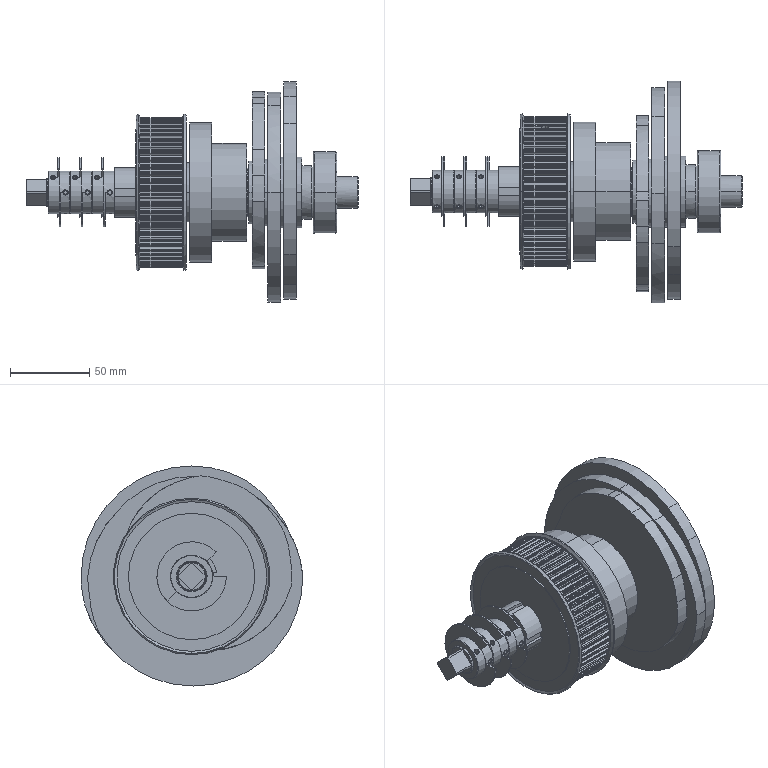Part | NX | 20 solids | 1082 faces | box 210 x 140.262 x 139.21 mm | volume 760392 mm3 | cylinder 733 | plane 222 | cone 74 | spline 29 | torus 24 | commonest cylinder face diameters 0.5 x124 1.1 x124 6.55 x124 94.53 x88 90.99 x63 2.5 x24